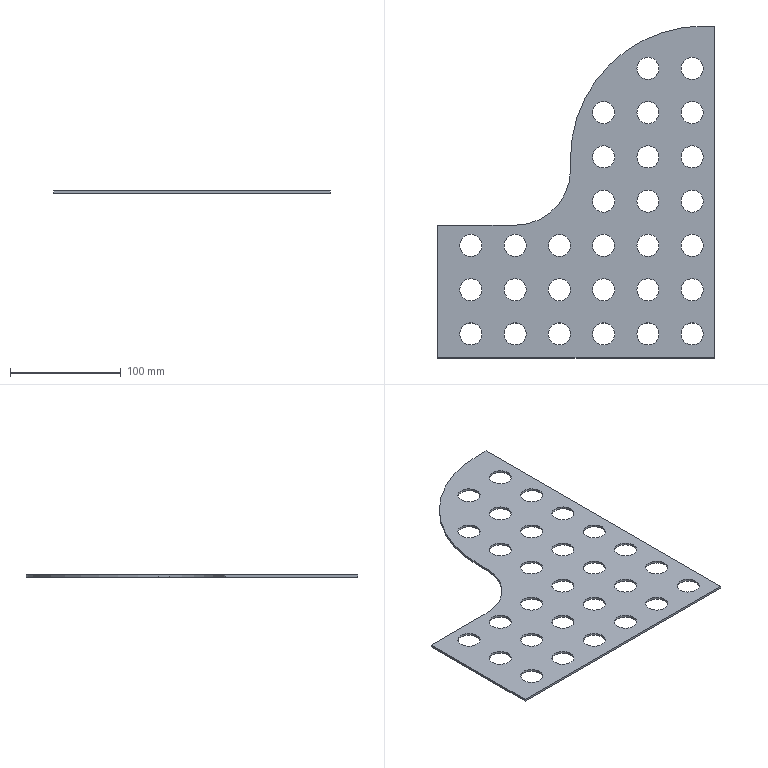Part | SolidWorks | features Extrusion 1, ICE 1 | 1 solid | 68 faces | box 250 x 300 x 2 mm | volume 83471 mm3 | cylinder 60 | plane 8 | commonest cylinder face diameters 20 x58 100 x1 240 x1